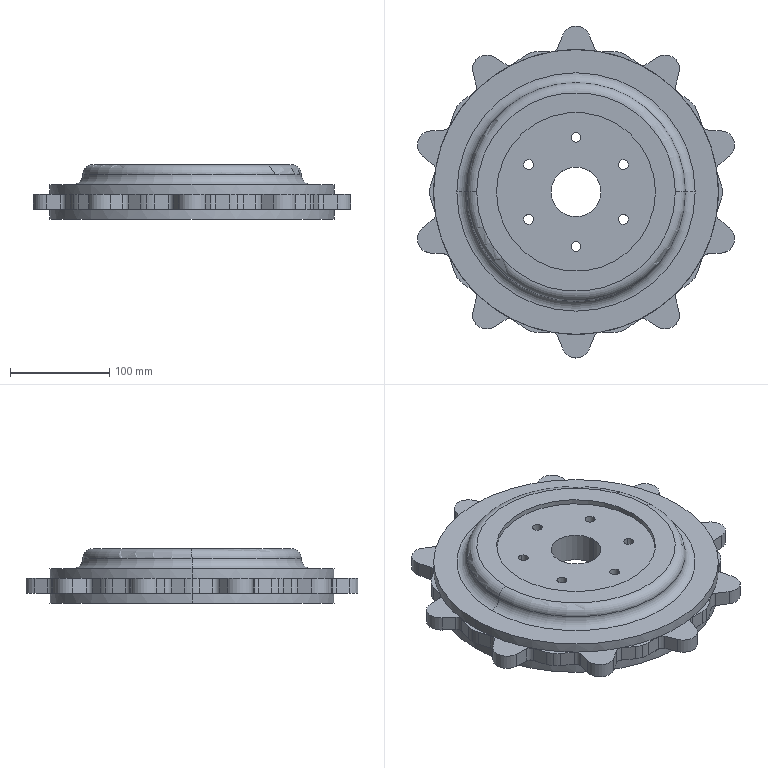Part | SolidWorks | features BaseBody 1 | 1 solid | 163 faces | box 319.348 x 334.309 x 55 mm | volume 2559395 mm3 | plane 85 | cylinder 70 | torus 8 | commonest cylinder face diameters 12 x20 48 x20 10 x12 28.63 x10 286.671 x4 50 x2